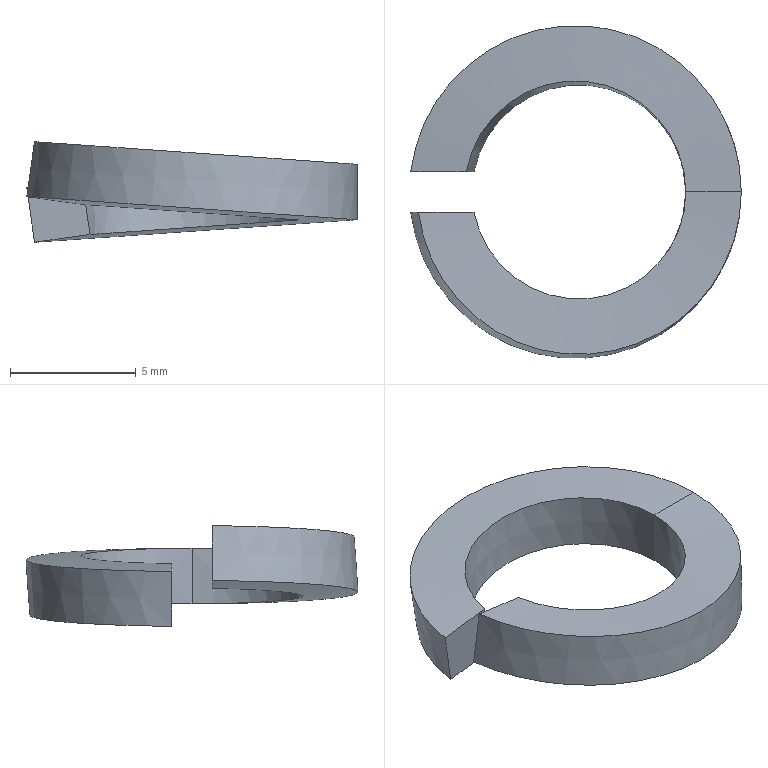Part | NX | features BREP 1 | 1 solid | 10 faces | box 13.121 x 13.202 x 3.992 mm | volume 157.257 mm3 | cone 8 | plane 2
STEP:
#1=CARTESIAN_POINT('',(-4.069,-0.8,2.788));
#2=VERTEX_POINT('',#1);
#3=CARTESIAN_POINT('',(-4.378,-0.8,0.6096));
#4=VERTEX_POINT('',#3);
#5=CARTESIAN_POINT('',(-4.069,-0.8,2.788));
#6=CARTESIAN_POINT('',(-4.114,-0.8,2.467));
#7=CARTESIAN_POINT('',(-4.16,-0.8,2.146));
#8=CARTESIAN_POINT('',(-4.256,-0.8,1.471));
#9=CARTESIAN_POINT('',(-4.306,-0.8,1.118));
#10=CARTESIAN_POINT('',(-4.363,-0.8,0.7125));
#11=CARTESIAN_POINT('',(-4.371,-0.8,0.661));
#12=CARTESIAN_POINT('',(-4.378,-0.8,0.6096));
#13=B_SPLINE_CURVE_WITH_KNOTS('',3,(#5,#6,#7,#8,#9,#10,#11,#12),.UNSPECIFIED.,.F.,.F.,(4,2,2,4),(0.,0.4421,0.9292,1.),.UNSPECIFIED.);
#14=EDGE_CURVE('',#2,#4,#13,.T.);
#15=ORIENTED_EDGE('',*,*,#14,.F.);
#16=CARTESIAN_POINT('',(4.34,0.,2.2));
#17=VERTEX_POINT('',#16);
#18=CARTESIAN_POINT('',(0.09766,0.,2.497));
#19=DIRECTION('',(0.06976,0.,0.9976));
#20=DIRECTION('',(0.9976,0.,-0.06976));
#21=AXIS2_PLACEMENT_3D('',#18,#19,#20);
#22=CIRCLE('',#21,4.253);
#23=EDGE_CURVE('',#2,#17,#22,.T.);
#24=ORIENTED_EDGE('',*,*,#23,.T.);
#25=CARTESIAN_POINT('',(4.34,0.,0.));
#26=VERTEX_POINT('',#25);
#27=CARTESIAN_POINT('',(4.34,0.,0.));
#28=DIRECTION('',(0.,0.,1.));
#29=VECTOR('',#28,1000.);
#30=LINE('',#27,#29);
#31=EDGE_CURVE('',#26,#17,#30,.T.);
#32=ORIENTED_EDGE('',*,*,#31,.F.);
#33=CARTESIAN_POINT('',(-0.05543,0.,0.3074));
#34=DIRECTION('',(0.06976,0.,0.9976));
#35=DIRECTION('',(0.9976,0.,-0.06976));
#36=AXIS2_PLACEMENT_3D('',#33,#34,#35);
#37=CIRCLE('',#36,4.406);
#38=EDGE_CURVE('',#4,#26,#37,.T.);
#39=ORIENTED_EDGE('',*,*,#38,.F.);
#40=EDGE_LOOP('',(#15,#24,#32,#39));
#41=FACE_BOUND('',#40,.T.);
#42=CARTESIAN_POINT('',(-0.05543,0.,0.3074));
#43=DIRECTION('',(-0.06976,0.,-0.9976));
#44=DIRECTION('',(0.9976,0.,-0.06976));
#45=AXIS2_PLACEMENT_3D('',#42,#43,#44);
#46=CONICAL_SURFACE('',#45,4.406,0.06981);
#47=ADVANCED_FACE('',(#41),#46,.F.);
#48=CARTESIAN_POINT('',(-6.274,-0.8,3.096));
#49=VERTEX_POINT('',#48);
#50=CARTESIAN_POINT('',(-6.274,-0.8,3.096));
#51=CARTESIAN_POINT('',(-5.539,-0.8,2.993));
#52=CARTESIAN_POINT('',(-4.804,-0.8,2.89));
#53=CARTESIAN_POINT('',(-4.069,-0.8,2.788));
#54=B_SPLINE_CURVE_WITH_KNOTS('',3,(#50,#51,#52,#53),.UNSPECIFIED.,.F.,.F.,(4,4),(0.,1.),.PIECEWISE_BEZIER_KNOTS.);
#55=EDGE_CURVE('',#49,#2,#54,.T.);
#56=ORIENTED_EDGE('',*,*,#55,.F.);
#57=CARTESIAN_POINT('',(6.54,0.,2.2));
#58=VERTEX_POINT('',#57);
#59=CARTESIAN_POINT('',(0.1084,0.,2.65));
#60=DIRECTION('',(0.06976,0.,0.9976));
#61=DIRECTION('',(0.9976,0.,-0.06976));
#62=AXIS2_PLACEMENT_3D('',#59,#60,#61);
#63=CIRCLE('',#62,6.447);
#64=EDGE_CURVE('',#49,#58,#63,.T.);
#65=ORIENTED_EDGE('',*,*,#64,.T.);
#66=CARTESIAN_POINT('',(4.34,0.,2.2));
#67=DIRECTION('',(1.,0.,0.));
#68=VECTOR('',#67,1000.);
#69=LINE('',#66,#68);
#70=EDGE_CURVE('',#17,#58,#69,.T.);
#71=ORIENTED_EDGE('',*,*,#70,.F.);
#72=ORIENTED_EDGE('',*,*,#23,.F.);
#73=EDGE_LOOP('',(#56,#65,#71,#72));
#74=FACE_BOUND('',#73,.T.);
#75=CARTESIAN_POINT('',(0.09766,0.,2.497));
#76=DIRECTION('',(0.06976,0.,0.9976));
#77=DIRECTION('',(-0.9976,0.,0.06976));
#78=AXIS2_PLACEMENT_3D('',#75,#76,#77);
#79=CONICAL_SURFACE('',#78,4.253,1.501);
#80=ADVANCED_FACE('',(#74),#79,.F.);
#81=CARTESIAN_POINT('',(-6.581,-0.8,0.9175));
#82=VERTEX_POINT('',#81);
#83=CARTESIAN_POINT('',(-6.581,-0.8,0.9175));
#84=CARTESIAN_POINT('',(-6.478,-0.8,1.644));
#85=CARTESIAN_POINT('',(-6.376,-0.8,2.37));
#86=CARTESIAN_POINT('',(-6.274,-0.8,3.096));
#87=B_SPLINE_CURVE_WITH_KNOTS('',3,(#83,#84,#85,#86),.UNSPECIFIED.,.F.,.F.,(4,4),(0.,1.),.PIECEWISE_BEZIER_KNOTS.);
#88=EDGE_CURVE('',#82,#49,#87,.T.);
#89=ORIENTED_EDGE('',*,*,#88,.F.);
#90=CARTESIAN_POINT('',(6.54,0.,0.));
#91=VERTEX_POINT('',#90);
#92=CARTESIAN_POINT('',(-0.04472,0.,0.4604));
#93=DIRECTION('',(0.06976,0.,0.9976));
#94=DIRECTION('',(0.9976,0.,-0.06976));
#95=AXIS2_PLACEMENT_3D('',#92,#93,#94);
#96=CIRCLE('',#95,6.601);
#97=EDGE_CURVE('',#82,#91,#96,.T.);
#98=ORIENTED_EDGE('',*,*,#97,.T.);
#99=CARTESIAN_POINT('',(6.54,0.,2.2));
#100=DIRECTION('',(0.,0.,-1.));
#101=VECTOR('',#100,1000.);
#102=LINE('',#99,#101);
#103=EDGE_CURVE('',#58,#91,#102,.T.);
#104=ORIENTED_EDGE('',*,*,#103,.F.);
#105=ORIENTED_EDGE('',*,*,#64,.F.);
#106=EDGE_LOOP('',(#89,#98,#104,#105));
#107=FACE_BOUND('',#106,.T.);
#108=CARTESIAN_POINT('',(0.1084,0.,2.65));
#109=DIRECTION('',(-0.06976,0.,-0.9976));
#110=DIRECTION('',(0.9976,0.,-0.06976));
#111=AXIS2_PLACEMENT_3D('',#108,#109,#110);
#112=CONICAL_SURFACE('',#111,6.447,0.06981);
#113=ADVANCED_FACE('',(#107),#112,.T.);
#114=CARTESIAN_POINT('',(-4.378,-0.8,0.6096));
#115=CARTESIAN_POINT('',(-5.112,-0.8,0.712));
#116=CARTESIAN_POINT('',(-5.847,-0.8,0.8147));
#117=CARTESIAN_POINT('',(-6.581,-0.8,0.9175));
#118=B_SPLINE_CURVE_WITH_KNOTS('',3,(#114,#115,#116,#117),.UNSPECIFIED.,.F.,.F.,(4,4),(0.,1.),.PIECEWISE_BEZIER_KNOTS.);
#119=EDGE_CURVE('',#4,#82,#118,.T.);
#120=ORIENTED_EDGE('',*,*,#119,.F.);
#121=ORIENTED_EDGE('',*,*,#38,.T.);
#122=CARTESIAN_POINT('',(6.54,0.,0.));
#123=DIRECTION('',(-1.,0.,0.));
#124=VECTOR('',#123,1000.);
#125=LINE('',#122,#124);
#126=EDGE_CURVE('',#91,#26,#125,.T.);
#127=ORIENTED_EDGE('',*,*,#126,.F.);
#128=ORIENTED_EDGE('',*,*,#97,.F.);
#129=EDGE_LOOP('',(#120,#121,#127,#128));
#130=FACE_BOUND('',#129,.T.);
#131=CARTESIAN_POINT('',(-0.04472,0.,0.4604));
#132=DIRECTION('',(0.06976,0.,0.9976));
#133=DIRECTION('',(-0.9976,0.,0.06976));
#134=AXIS2_PLACEMENT_3D('',#131,#132,#133);
#135=CONICAL_SURFACE('',#134,6.601,1.501);
#136=ADVANCED_FACE('',(#130),#135,.T.);
#137=CARTESIAN_POINT('',(-4.378,0.8,1.59));
#138=VERTEX_POINT('',#137);
#139=CARTESIAN_POINT('',(-0.05543,0.,1.893));
#140=DIRECTION('',(0.06976,0.,-0.9976));
#141=DIRECTION('',(-0.9976,0.,-0.06976));
#142=AXIS2_PLACEMENT_3D('',#139,#140,#141);
#143=CIRCLE('',#142,4.406);
#144=EDGE_CURVE('',#138,#17,#143,.T.);
#145=ORIENTED_EDGE('',*,*,#144,.F.);
#146=CARTESIAN_POINT('',(-4.069,0.8,-0.588));
#147=VERTEX_POINT('',#146);
#148=CARTESIAN_POINT('',(-4.378,0.8,1.59));
#149=CARTESIAN_POINT('',(-4.306,0.8,1.083));
#150=CARTESIAN_POINT('',(-4.234,0.8,0.5748));
#151=CARTESIAN_POINT('',(-4.131,0.8,-0.1513));
#152=CARTESIAN_POINT('',(-4.1,0.8,-0.3697));
#153=CARTESIAN_POINT('',(-4.069,0.8,-0.588));
#154=B_SPLINE_CURVE_WITH_KNOTS('',3,(#148,#149,#150,#151,#152,#153),.UNSPECIFIED.,.F.,.F.,(4,2,4),(0.,0.6993,1.),.UNSPECIFIED.);
#155=EDGE_CURVE('',#138,#147,#154,.T.);
#156=ORIENTED_EDGE('',*,*,#155,.T.);
#157=CARTESIAN_POINT('',(0.09766,0.,-0.2967));
#158=DIRECTION('',(0.06976,0.,-0.9976));
#159=DIRECTION('',(-0.9976,0.,-0.06976));
#160=AXIS2_PLACEMENT_3D('',#157,#158,#159);
#161=CIRCLE('',#160,4.253);
#162=EDGE_CURVE('',#147,#26,#161,.T.);
#163=ORIENTED_EDGE('',*,*,#162,.T.);
#164=ORIENTED_EDGE('',*,*,#31,.T.);
#165=EDGE_LOOP('',(#145,#156,#163,#164));
#166=FACE_BOUND('',#165,.T.);
#167=CARTESIAN_POINT('',(0.09766,0.,-0.2967));
#168=DIRECTION('',(-0.06976,0.,0.9976));
#169=DIRECTION('',(-0.9976,0.,-0.06976));
#170=AXIS2_PLACEMENT_3D('',#167,#168,#169);
#171=CONICAL_SURFACE('',#170,4.253,0.06981);
#172=ADVANCED_FACE('',(#166),#171,.F.);
#173=CARTESIAN_POINT('',(-6.581,0.8,1.282));
#174=VERTEX_POINT('',#173);
#175=CARTESIAN_POINT('',(-0.04472,0.,1.74));
#176=DIRECTION('',(0.06976,0.,-0.9976));
#177=DIRECTION('',(-0.9976,0.,-0.06976));
#178=AXIS2_PLACEMENT_3D('',#175,#176,#177);
#179=CIRCLE('',#178,6.601);
#180=EDGE_CURVE('',#174,#58,#179,.T.);
#181=ORIENTED_EDGE('',*,*,#180,.F.);
#182=CARTESIAN_POINT('',(-6.581,0.8,1.282));
#183=CARTESIAN_POINT('',(-5.847,0.8,1.385));
#184=CARTESIAN_POINT('',(-5.112,0.8,1.488));
#185=CARTESIAN_POINT('',(-4.378,0.8,1.59));
#186=B_SPLINE_CURVE_WITH_KNOTS('',3,(#182,#183,#184,#185),.UNSPECIFIED.,.F.,.F.,(4,4),(0.,1.),.PIECEWISE_BEZIER_KNOTS.);
#187=EDGE_CURVE('',#174,#138,#186,.T.);
#188=ORIENTED_EDGE('',*,*,#187,.T.);
#189=ORIENTED_EDGE('',*,*,#144,.T.);
#190=ORIENTED_EDGE('',*,*,#70,.T.);
#191=EDGE_LOOP('',(#181,#188,#189,#190));
#192=FACE_BOUND('',#191,.T.);
#193=CARTESIAN_POINT('',(-0.05543,0.,1.893));
#194=DIRECTION('',(0.06976,0.,-0.9976));
#195=DIRECTION('',(0.9976,0.,0.06976));
#196=AXIS2_PLACEMENT_3D('',#193,#194,#195);
#197=CONICAL_SURFACE('',#196,4.406,1.501);
#198=ADVANCED_FACE('',(#192),#197,.T.);
#199=CARTESIAN_POINT('',(-6.274,0.8,-0.896));
#200=VERTEX_POINT('',#199);
#201=CARTESIAN_POINT('',(0.1084,0.,-0.4497));
#202=DIRECTION('',(0.06976,0.,-0.9976));
#203=DIRECTION('',(-0.9976,0.,-0.06976));
#204=AXIS2_PLACEMENT_3D('',#201,#202,#203);
#205=CIRCLE('',#204,6.447);
#206=EDGE_CURVE('',#200,#91,#205,.T.);
#207=ORIENTED_EDGE('',*,*,#206,.F.);
#208=CARTESIAN_POINT('',(-6.274,0.8,-0.896));
#209=CARTESIAN_POINT('',(-6.306,0.8,-0.6657));
#210=CARTESIAN_POINT('',(-6.339,0.8,-0.4354));
#211=CARTESIAN_POINT('',(-6.441,0.8,0.2907));
#212=CARTESIAN_POINT('',(-6.511,0.8,0.7866));
#213=CARTESIAN_POINT('',(-6.581,0.8,1.282));
#214=B_SPLINE_CURVE_WITH_KNOTS('',3,(#208,#209,#210,#211,#212,#213),.UNSPECIFIED.,.F.,.F.,(4,2,4),(0.,0.3171,1.),.UNSPECIFIED.);
#215=EDGE_CURVE('',#200,#174,#214,.T.);
#216=ORIENTED_EDGE('',*,*,#215,.T.);
#217=ORIENTED_EDGE('',*,*,#180,.T.);
#218=ORIENTED_EDGE('',*,*,#103,.T.);
#219=EDGE_LOOP('',(#207,#216,#217,#218));
#220=FACE_BOUND('',#219,.T.);
#221=CARTESIAN_POINT('',(-0.04472,0.,1.74));
#222=DIRECTION('',(-0.06976,0.,0.9976));
#223=DIRECTION('',(-0.9976,0.,-0.06976));
#224=AXIS2_PLACEMENT_3D('',#221,#222,#223);
#225=CONICAL_SURFACE('',#224,6.601,0.06981);
#226=ADVANCED_FACE('',(#220),#225,.T.);
#227=ORIENTED_EDGE('',*,*,#162,.F.);
#228=CARTESIAN_POINT('',(-4.069,0.8,-0.588));
#229=CARTESIAN_POINT('',(-4.804,0.8,-0.6904));
#230=CARTESIAN_POINT('',(-5.539,0.8,-0.7931));
#231=CARTESIAN_POINT('',(-6.274,0.8,-0.896));
#232=B_SPLINE_CURVE_WITH_KNOTS('',3,(#228,#229,#230,#231),.UNSPECIFIED.,.F.,.F.,(4,4),(0.,1.),.PIECEWISE_BEZIER_KNOTS.);
#233=EDGE_CURVE('',#147,#200,#232,.T.);
#234=ORIENTED_EDGE('',*,*,#233,.T.);
#235=ORIENTED_EDGE('',*,*,#206,.T.);
#236=ORIENTED_EDGE('',*,*,#126,.T.);
#237=EDGE_LOOP('',(#227,#234,#235,#236));
#238=FACE_BOUND('',#237,.T.);
#239=CARTESIAN_POINT('',(0.1084,0.,-0.4497));
#240=DIRECTION('',(0.06976,0.,-0.9976));
#241=DIRECTION('',(0.9976,0.,0.06976));
#242=AXIS2_PLACEMENT_3D('',#239,#240,#241);
#243=CONICAL_SURFACE('',#242,6.447,1.501);
#244=ADVANCED_FACE('',(#238),#243,.F.);
#245=ORIENTED_EDGE('',*,*,#187,.F.);
#246=ORIENTED_EDGE('',*,*,#215,.F.);
#247=ORIENTED_EDGE('',*,*,#233,.F.);
#248=ORIENTED_EDGE('',*,*,#155,.F.);
#249=EDGE_LOOP('',(#245,#246,#247,#248));
#250=FACE_BOUND('',#249,.T.);
#251=CARTESIAN_POINT('',(0.,0.8,-13.08));
#252=DIRECTION('',(0.,1.,0.));
#253=DIRECTION('',(0.,0.,-1.));
#254=AXIS2_PLACEMENT_3D('',#251,#252,#253);
#255=PLANE('',#254);
#256=ADVANCED_FACE('',(#250),#255,.F.);
#257=ORIENTED_EDGE('',*,*,#14,.T.);
#258=ORIENTED_EDGE('',*,*,#119,.T.);
#259=ORIENTED_EDGE('',*,*,#88,.T.);
#260=ORIENTED_EDGE('',*,*,#55,.T.);
#261=EDGE_LOOP('',(#257,#258,#259,#260));
#262=FACE_BOUND('',#261,.T.);
#263=CARTESIAN_POINT('',(-13.08,-0.8,-13.08));
#264=DIRECTION('',(0.,-1.,0.));
#265=DIRECTION('',(0.,0.,1.));
#266=AXIS2_PLACEMENT_3D('',#263,#264,#265);
#267=PLANE('',#266);
#268=ADVANCED_FACE('',(#262),#267,.F.);
#269=CLOSED_SHELL('',(#47,#80,#113,#136,#172,#198,#226,#244,#256,#268));
#270=MANIFOLD_SOLID_BREP('',#269);
#271=(LENGTH_UNIT()NAMED_UNIT(*)SI_UNIT(.MILLI.,.METRE.));
#272=UNCERTAINTY_MEASURE_WITH_UNIT(LENGTH_MEASURE(0.00001),#271,'','');
#273=(NAMED_UNIT(*)PLANE_ANGLE_UNIT()SI_UNIT($,.RADIAN.));
#274=(NAMED_UNIT(*)SI_UNIT($,.STERADIAN.)SOLID_ANGLE_UNIT());
#275=(GEOMETRIC_REPRESENTATION_CONTEXT(3)GLOBAL_UNCERTAINTY_ASSIGNED_CONTEXT((#272))GLOBAL_UNIT_ASSIGNED_CONTEXT((#271,#273,#274))REPRESENTATION_CONTEXT('',''));
#276=ADVANCED_BREP_SHAPE_REPRESENTATION('',(#270),#275);